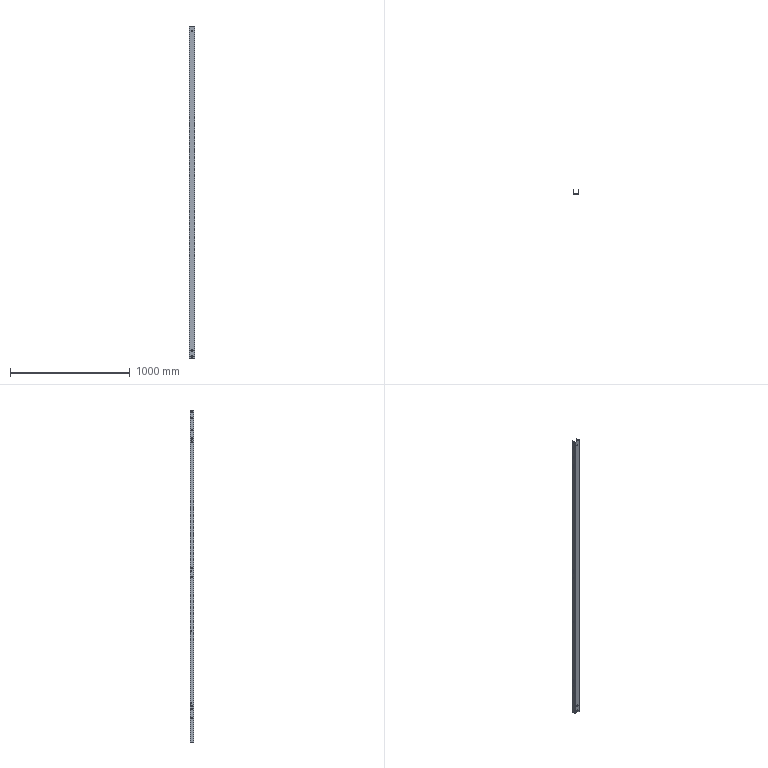Part | SolidWorks | features ICE 2, FlatPattern 1, SMBaseFlange 1, SheetMetal 1 | 1 solid | 80 faces | box 50 x 30 x 2775 mm | volume 844323 mm3 | cylinder 62 | plane 18 | commonest cylinder face diameters 11 x32 10 x12 13 x10 17 x4 0.4 x2 6.4 x2